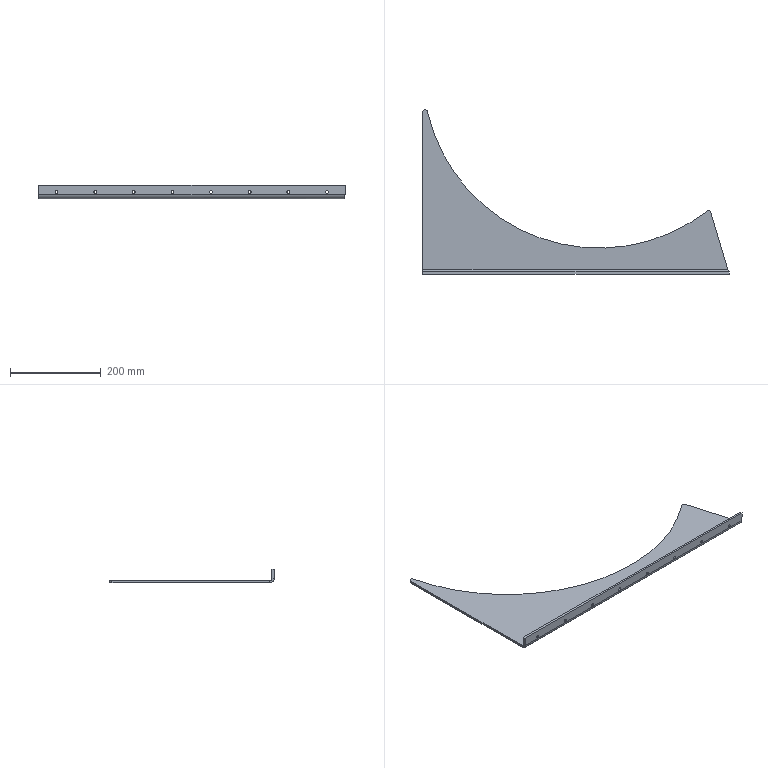Part | SolidWorks | features EdgeFlange 1, Fillet 1, FlatPattern 1, HoleWzd 1, LPattern 1, SMBaseFlange 1, SheetMetal 1 | 1 solid | 48 faces | box 673.852 x 361.966 x 30 mm | volume 462182 mm3 | cylinder 21 | cone 16 | plane 10 | spline 1 | commonest cylinder face diameters 6 x16 10 x3 20 x1 775 x1
STEP:
#1=CARTESIAN_POINT('',(161.352,-444.975,18.));
#2=VERTEX_POINT('',#1);
#3=CARTESIAN_POINT('',(161.352,-444.975,12.));
#4=VERTEX_POINT('',#3);
#5=CARTESIAN_POINT('',(161.352,-444.975,15.));
#6=DIRECTION('',(0.,-1.,0.));
#7=DIRECTION('',(0.,0.,-1.));
#8=AXIS2_PLACEMENT_3D('',#5,#6,#7);
#9=CIRCLE('',#8,3.);
#10=EDGE_CURVE('',#2,#4,#9,.T.);
#11=ORIENTED_EDGE('',*,*,#10,.F.);
#12=CARTESIAN_POINT('',(161.352,-445.,18.025));
#13=VERTEX_POINT('',#12);
#14=CARTESIAN_POINT('',(161.352,-445.,18.025));
#15=DIRECTION('',(0.,-0.7071,0.7071));
#16=VECTOR('',#15,1000.);
#17=LINE('',#14,#16);
#18=EDGE_CURVE('',#2,#13,#17,.T.);
#19=ORIENTED_EDGE('',*,*,#18,.T.);
#20=CARTESIAN_POINT('',(161.352,-445.,11.975));
#21=VERTEX_POINT('',#20);
#22=CARTESIAN_POINT('',(161.352,-445.,15.));
#23=DIRECTION('',(0.,-1.,0.));
#24=DIRECTION('',(0.,0.,-1.));
#25=AXIS2_PLACEMENT_3D('',#22,#23,#24);
#26=CIRCLE('',#25,3.025);
#27=EDGE_CURVE('',#13,#21,#26,.T.);
#28=ORIENTED_EDGE('',*,*,#27,.T.);
#29=CARTESIAN_POINT('',(161.352,-445.,11.975));
#30=DIRECTION('',(0.,-0.7071,-0.7071));
#31=VECTOR('',#30,1000.);
#32=LINE('',#29,#31);
#33=EDGE_CURVE('',#4,#21,#32,.T.);
#34=ORIENTED_EDGE('',*,*,#33,.F.);
#35=EDGE_LOOP('',(#11,#19,#28,#34));
#36=FACE_OUTER_BOUND('',#35,.T.);
#37=CARTESIAN_POINT('',(161.352,-445.,15.));
#38=DIRECTION('',(0.,-1.,0.));
#39=DIRECTION('',(0.,0.,-1.));
#40=AXIS2_PLACEMENT_3D('',#37,#38,#39);
#41=CONICAL_SURFACE('',#40,3.025,0.7854);
#42=ADVANCED_FACE('',(#36),#41,.F.);
#43=CARTESIAN_POINT('',(161.352,-440.,18.));
#44=VERTEX_POINT('',#43);
#45=CARTESIAN_POINT('',(161.352,-440.,12.));
#46=VERTEX_POINT('',#45);
#47=CARTESIAN_POINT('',(161.352,-440.,15.));
#48=DIRECTION('',(0.,-1.,0.));
#49=DIRECTION('',(0.,0.,-1.));
#50=AXIS2_PLACEMENT_3D('',#47,#48,#49);
#51=CIRCLE('',#50,3.);
#52=EDGE_CURVE('',#44,#46,#51,.T.);
#53=ORIENTED_EDGE('',*,*,#52,.F.);
#54=CARTESIAN_POINT('',(161.352,-445.,18.));
#55=DIRECTION('',(0.,-1.,0.));
#56=VECTOR('',#55,1000.);
#57=LINE('',#54,#56);
#58=EDGE_CURVE('',#44,#2,#57,.T.);
#59=ORIENTED_EDGE('',*,*,#58,.T.);
#60=ORIENTED_EDGE('',*,*,#10,.T.);
#61=CARTESIAN_POINT('',(161.352,-445.,12.));
#62=DIRECTION('',(0.,-1.,0.));
#63=VECTOR('',#62,1000.);
#64=LINE('',#61,#63);
#65=EDGE_CURVE('',#46,#4,#64,.T.);
#66=ORIENTED_EDGE('',*,*,#65,.F.);
#67=EDGE_LOOP('',(#53,#59,#60,#66));
#68=FACE_OUTER_BOUND('',#67,.T.);
#69=CARTESIAN_POINT('',(161.352,-445.,15.));
#70=DIRECTION('',(0.,-1.,0.));
#71=DIRECTION('',(0.,0.,-1.));
#72=AXIS2_PLACEMENT_3D('',#69,#70,#71);
#73=CYLINDRICAL_SURFACE('',#72,3.);
#74=ADVANCED_FACE('',(#68),#73,.F.);
#75=CARTESIAN_POINT('',(246.352,-444.975,18.));
#76=VERTEX_POINT('',#75);
#77=CARTESIAN_POINT('',(246.352,-444.975,12.));
#78=VERTEX_POINT('',#77);
#79=CARTESIAN_POINT('',(246.352,-444.975,15.));
#80=DIRECTION('',(0.,-1.,0.));
#81=DIRECTION('',(0.,0.,-1.));
#82=AXIS2_PLACEMENT_3D('',#79,#80,#81);
#83=CIRCLE('',#82,3.);
#84=EDGE_CURVE('',#76,#78,#83,.T.);
#85=ORIENTED_EDGE('',*,*,#84,.F.);
#86=CARTESIAN_POINT('',(246.352,-445.,18.025));
#87=VERTEX_POINT('',#86);
#88=CARTESIAN_POINT('',(246.352,-445.,18.025));
#89=DIRECTION('',(0.,-0.7071,0.7071));
#90=VECTOR('',#89,1000.);
#91=LINE('',#88,#90);
#92=EDGE_CURVE('',#76,#87,#91,.T.);
#93=ORIENTED_EDGE('',*,*,#92,.T.);
#94=CARTESIAN_POINT('',(246.352,-445.,11.975));
#95=VERTEX_POINT('',#94);
#96=CARTESIAN_POINT('',(246.352,-445.,15.));
#97=DIRECTION('',(0.,-1.,0.));
#98=DIRECTION('',(0.,0.,-1.));
#99=AXIS2_PLACEMENT_3D('',#96,#97,#98);
#100=CIRCLE('',#99,3.025);
#101=EDGE_CURVE('',#87,#95,#100,.T.);
#102=ORIENTED_EDGE('',*,*,#101,.T.);
#103=CARTESIAN_POINT('',(246.352,-445.,11.975));
#104=DIRECTION('',(0.,-0.7071,-0.7071));
#105=VECTOR('',#104,1000.);
#106=LINE('',#103,#105);
#107=EDGE_CURVE('',#78,#95,#106,.T.);
#108=ORIENTED_EDGE('',*,*,#107,.F.);
#109=EDGE_LOOP('',(#85,#93,#102,#108));
#110=FACE_OUTER_BOUND('',#109,.T.);
#111=CARTESIAN_POINT('',(246.352,-445.,15.));
#112=DIRECTION('',(0.,-1.,0.));
#113=DIRECTION('',(0.,0.,-1.));
#114=AXIS2_PLACEMENT_3D('',#111,#112,#113);
#115=CONICAL_SURFACE('',#114,3.025,0.7854);
#116=ADVANCED_FACE('',(#110),#115,.F.);
#117=CARTESIAN_POINT('',(246.352,-440.,18.));
#118=VERTEX_POINT('',#117);
#119=CARTESIAN_POINT('',(246.352,-440.,12.));
#120=VERTEX_POINT('',#119);
#121=CARTESIAN_POINT('',(246.352,-440.,15.));
#122=DIRECTION('',(0.,-1.,0.));
#123=DIRECTION('',(0.,0.,-1.));
#124=AXIS2_PLACEMENT_3D('',#121,#122,#123);
#125=CIRCLE('',#124,3.);
#126=EDGE_CURVE('',#118,#120,#125,.T.);
#127=ORIENTED_EDGE('',*,*,#126,.F.);
#128=CARTESIAN_POINT('',(246.352,-445.,18.));
#129=DIRECTION('',(0.,-1.,0.));
#130=VECTOR('',#129,1000.);
#131=LINE('',#128,#130);
#132=EDGE_CURVE('',#118,#76,#131,.T.);
#133=ORIENTED_EDGE('',*,*,#132,.T.);
#134=ORIENTED_EDGE('',*,*,#84,.T.);
#135=CARTESIAN_POINT('',(246.352,-445.,12.));
#136=DIRECTION('',(0.,-1.,0.));
#137=VECTOR('',#136,1000.);
#138=LINE('',#135,#137);
#139=EDGE_CURVE('',#120,#78,#138,.T.);
#140=ORIENTED_EDGE('',*,*,#139,.F.);
#141=EDGE_LOOP('',(#127,#133,#134,#140));
#142=FACE_OUTER_BOUND('',#141,.T.);
#143=CARTESIAN_POINT('',(246.352,-445.,15.));
#144=DIRECTION('',(0.,-1.,0.));
#145=DIRECTION('',(0.,0.,-1.));
#146=AXIS2_PLACEMENT_3D('',#143,#144,#145);
#147=CYLINDRICAL_SURFACE('',#146,3.);
#148=ADVANCED_FACE('',(#142),#147,.F.);
#149=CARTESIAN_POINT('',(76.352,-440.,18.));
#150=VERTEX_POINT('',#149);
#151=CARTESIAN_POINT('',(76.352,-440.,12.));
#152=VERTEX_POINT('',#151);
#153=CARTESIAN_POINT('',(76.352,-440.,15.));
#154=DIRECTION('',(0.,-1.,0.));
#155=DIRECTION('',(0.,0.,-1.));
#156=AXIS2_PLACEMENT_3D('',#153,#154,#155);
#157=CIRCLE('',#156,3.);
#158=EDGE_CURVE('',#150,#152,#157,.T.);
#159=ORIENTED_EDGE('',*,*,#158,.F.);
#160=CARTESIAN_POINT('',(76.352,-444.975,18.));
#161=VERTEX_POINT('',#160);
#162=CARTESIAN_POINT('',(76.352,-445.,18.));
#163=DIRECTION('',(0.,-1.,0.));
#164=VECTOR('',#163,1000.);
#165=LINE('',#162,#164);
#166=EDGE_CURVE('',#150,#161,#165,.T.);
#167=ORIENTED_EDGE('',*,*,#166,.T.);
#168=CARTESIAN_POINT('',(76.352,-444.975,12.));
#169=VERTEX_POINT('',#168);
#170=CARTESIAN_POINT('',(76.352,-444.975,15.));
#171=DIRECTION('',(0.,-1.,0.));
#172=DIRECTION('',(0.,0.,-1.));
#173=AXIS2_PLACEMENT_3D('',#170,#171,#172);
#174=CIRCLE('',#173,3.);
#175=EDGE_CURVE('',#161,#169,#174,.T.);
#176=ORIENTED_EDGE('',*,*,#175,.T.);
#177=CARTESIAN_POINT('',(76.352,-445.,12.));
#178=DIRECTION('',(0.,-1.,0.));
#179=VECTOR('',#178,1000.);
#180=LINE('',#177,#179);
#181=EDGE_CURVE('',#152,#169,#180,.T.);
#182=ORIENTED_EDGE('',*,*,#181,.F.);
#183=EDGE_LOOP('',(#159,#167,#176,#182));
#184=FACE_OUTER_BOUND('',#183,.T.);
#185=CARTESIAN_POINT('',(76.352,-445.,15.));
#186=DIRECTION('',(0.,-1.,0.));
#187=DIRECTION('',(0.,0.,-1.));
#188=AXIS2_PLACEMENT_3D('',#185,#186,#187);
#189=CYLINDRICAL_SURFACE('',#188,3.);
#190=ADVANCED_FACE('',(#184),#189,.F.);
#191=ORIENTED_EDGE('',*,*,#175,.F.);
#192=CARTESIAN_POINT('',(76.352,-445.,18.025));
#193=VERTEX_POINT('',#192);
#194=CARTESIAN_POINT('',(76.352,-445.,18.025));
#195=DIRECTION('',(0.,-0.7071,0.7071));
#196=VECTOR('',#195,1000.);
#197=LINE('',#194,#196);
#198=EDGE_CURVE('',#161,#193,#197,.T.);
#199=ORIENTED_EDGE('',*,*,#198,.T.);
#200=CARTESIAN_POINT('',(76.352,-445.,11.975));
#201=VERTEX_POINT('',#200);
#202=CARTESIAN_POINT('',(76.352,-445.,15.));
#203=DIRECTION('',(0.,-1.,0.));
#204=DIRECTION('',(0.,0.,-1.));
#205=AXIS2_PLACEMENT_3D('',#202,#203,#204);
#206=CIRCLE('',#205,3.025);
#207=EDGE_CURVE('',#193,#201,#206,.T.);
#208=ORIENTED_EDGE('',*,*,#207,.T.);
#209=CARTESIAN_POINT('',(76.352,-445.,11.975));
#210=DIRECTION('',(0.,-0.7071,-0.7071));
#211=VECTOR('',#210,1000.);
#212=LINE('',#209,#211);
#213=EDGE_CURVE('',#169,#201,#212,.T.);
#214=ORIENTED_EDGE('',*,*,#213,.F.);
#215=EDGE_LOOP('',(#191,#199,#208,#214));
#216=FACE_OUTER_BOUND('',#215,.T.);
#217=CARTESIAN_POINT('',(76.352,-445.,15.));
#218=DIRECTION('',(0.,-1.,0.));
#219=DIRECTION('',(0.,0.,-1.));
#220=AXIS2_PLACEMENT_3D('',#217,#218,#219);
#221=CONICAL_SURFACE('',#220,3.025,0.7854);
#222=ADVANCED_FACE('',(#216),#221,.F.);
#223=CARTESIAN_POINT('',(-8.648,-440.,18.));
#224=VERTEX_POINT('',#223);
#225=CARTESIAN_POINT('',(-8.648,-440.,12.));
#226=VERTEX_POINT('',#225);
#227=CARTESIAN_POINT('',(-8.648,-440.,15.));
#228=DIRECTION('',(0.,-1.,0.));
#229=DIRECTION('',(0.,0.,-1.));
#230=AXIS2_PLACEMENT_3D('',#227,#228,#229);
#231=CIRCLE('',#230,3.);
#232=EDGE_CURVE('',#224,#226,#231,.T.);
#233=ORIENTED_EDGE('',*,*,#232,.F.);
#234=CARTESIAN_POINT('',(-8.648,-444.975,18.));
#235=VERTEX_POINT('',#234);
#236=CARTESIAN_POINT('',(-8.648,-445.,18.));
#237=DIRECTION('',(0.,-1.,0.));
#238=VECTOR('',#237,1000.);
#239=LINE('',#236,#238);
#240=EDGE_CURVE('',#224,#235,#239,.T.);
#241=ORIENTED_EDGE('',*,*,#240,.T.);
#242=CARTESIAN_POINT('',(-8.648,-444.975,12.));
#243=VERTEX_POINT('',#242);
#244=CARTESIAN_POINT('',(-8.648,-444.975,15.));
#245=DIRECTION('',(0.,-1.,0.));
#246=DIRECTION('',(0.,0.,-1.));
#247=AXIS2_PLACEMENT_3D('',#244,#245,#246);
#248=CIRCLE('',#247,3.);
#249=EDGE_CURVE('',#235,#243,#248,.T.);
#250=ORIENTED_EDGE('',*,*,#249,.T.);
#251=CARTESIAN_POINT('',(-8.648,-445.,12.));
#252=DIRECTION('',(0.,-1.,0.));
#253=VECTOR('',#252,1000.);
#254=LINE('',#251,#253);
#255=EDGE_CURVE('',#226,#243,#254,.T.);
#256=ORIENTED_EDGE('',*,*,#255,.F.);
#257=EDGE_LOOP('',(#233,#241,#250,#256));
#258=FACE_OUTER_BOUND('',#257,.T.);
#259=CARTESIAN_POINT('',(-8.648,-445.,15.));
#260=DIRECTION('',(0.,-1.,0.));
#261=DIRECTION('',(0.,0.,-1.));
#262=AXIS2_PLACEMENT_3D('',#259,#260,#261);
#263=CYLINDRICAL_SURFACE('',#262,3.);
#264=ADVANCED_FACE('',(#258),#263,.F.);
#265=ORIENTED_EDGE('',*,*,#249,.F.);
#266=CARTESIAN_POINT('',(-8.648,-445.,18.025));
#267=VERTEX_POINT('',#266);
#268=CARTESIAN_POINT('',(-8.648,-445.,18.025));
#269=DIRECTION('',(0.,-0.7071,0.7071));
#270=VECTOR('',#269,1000.);
#271=LINE('',#268,#270);
#272=EDGE_CURVE('',#235,#267,#271,.T.);
#273=ORIENTED_EDGE('',*,*,#272,.T.);
#274=CARTESIAN_POINT('',(-8.648,-445.,11.975));
#275=VERTEX_POINT('',#274);
#276=CARTESIAN_POINT('',(-8.648,-445.,15.));
#277=DIRECTION('',(0.,-1.,0.));
#278=DIRECTION('',(0.,0.,-1.));
#279=AXIS2_PLACEMENT_3D('',#276,#277,#278);
#280=CIRCLE('',#279,3.025);
#281=EDGE_CURVE('',#267,#275,#280,.T.);
#282=ORIENTED_EDGE('',*,*,#281,.T.);
#283=CARTESIAN_POINT('',(-8.648,-445.,11.975));
#284=DIRECTION('',(0.,-0.7071,-0.7071));
#285=VECTOR('',#284,1000.);
#286=LINE('',#283,#285);
#287=EDGE_CURVE('',#243,#275,#286,.T.);
#288=ORIENTED_EDGE('',*,*,#287,.F.);
#289=EDGE_LOOP('',(#265,#273,#282,#288));
#290=FACE_OUTER_BOUND('',#289,.T.);
#291=CARTESIAN_POINT('',(-8.648,-445.,15.));
#292=DIRECTION('',(0.,-1.,0.));
#293=DIRECTION('',(0.,0.,-1.));
#294=AXIS2_PLACEMENT_3D('',#291,#292,#293);
#295=CONICAL_SURFACE('',#294,3.025,0.7854);
#296=ADVANCED_FACE('',(#290),#295,.F.);
#297=CARTESIAN_POINT('',(-93.648,-440.,18.));
#298=VERTEX_POINT('',#297);
#299=CARTESIAN_POINT('',(-93.648,-440.,12.));
#300=VERTEX_POINT('',#299);
#301=CARTESIAN_POINT('',(-93.648,-440.,15.));
#302=DIRECTION('',(0.,-1.,0.));
#303=DIRECTION('',(0.,0.,-1.));
#304=AXIS2_PLACEMENT_3D('',#301,#302,#303);
#305=CIRCLE('',#304,3.);
#306=EDGE_CURVE('',#298,#300,#305,.T.);
#307=ORIENTED_EDGE('',*,*,#306,.F.);
#308=CARTESIAN_POINT('',(-93.648,-444.975,18.));
#309=VERTEX_POINT('',#308);
#310=CARTESIAN_POINT('',(-93.648,-445.,18.));
#311=DIRECTION('',(0.,-1.,0.));
#312=VECTOR('',#311,1000.);
#313=LINE('',#310,#312);
#314=EDGE_CURVE('',#298,#309,#313,.T.);
#315=ORIENTED_EDGE('',*,*,#314,.T.);
#316=CARTESIAN_POINT('',(-93.648,-444.975,12.));
#317=VERTEX_POINT('',#316);
#318=CARTESIAN_POINT('',(-93.648,-444.975,15.));
#319=DIRECTION('',(0.,-1.,0.));
#320=DIRECTION('',(0.,0.,-1.));
#321=AXIS2_PLACEMENT_3D('',#318,#319,#320);
#322=CIRCLE('',#321,3.);
#323=EDGE_CURVE('',#309,#317,#322,.T.);
#324=ORIENTED_EDGE('',*,*,#323,.T.);
#325=CARTESIAN_POINT('',(-93.648,-445.,12.));
#326=DIRECTION('',(0.,-1.,0.));
#327=VECTOR('',#326,1000.);
#328=LINE('',#325,#327);
#329=EDGE_CURVE('',#300,#317,#328,.T.);
#330=ORIENTED_EDGE('',*,*,#329,.F.);
#331=EDGE_LOOP('',(#307,#315,#324,#330));
#332=FACE_OUTER_BOUND('',#331,.T.);
#333=CARTESIAN_POINT('',(-93.648,-445.,15.));
#334=DIRECTION('',(0.,-1.,0.));
#335=DIRECTION('',(0.,0.,-1.));
#336=AXIS2_PLACEMENT_3D('',#333,#334,#335);
#337=CYLINDRICAL_SURFACE('',#336,3.);
#338=ADVANCED_FACE('',(#332),#337,.F.);
#339=ORIENTED_EDGE('',*,*,#323,.F.);
#340=CARTESIAN_POINT('',(-93.648,-445.,18.025));
#341=VERTEX_POINT('',#340);
#342=CARTESIAN_POINT('',(-93.648,-445.,18.025));
#343=DIRECTION('',(0.,-0.7071,0.7071));
#344=VECTOR('',#343,1000.);
#345=LINE('',#342,#344);
#346=EDGE_CURVE('',#309,#341,#345,.T.);
#347=ORIENTED_EDGE('',*,*,#346,.T.);
#348=CARTESIAN_POINT('',(-93.648,-445.,11.975));
#349=VERTEX_POINT('',#348);
#350=CARTESIAN_POINT('',(-93.648,-445.,15.));
#351=DIRECTION('',(0.,-1.,0.));
#352=DIRECTION('',(0.,0.,-1.));
#353=AXIS2_PLACEMENT_3D('',#350,#351,#352);
#354=CIRCLE('',#353,3.025);
#355=EDGE_CURVE('',#341,#349,#354,.T.);
#356=ORIENTED_EDGE('',*,*,#355,.T.);
#357=CARTESIAN_POINT('',(-93.648,-445.,11.975));
#358=DIRECTION('',(0.,-0.7071,-0.7071));
#359=VECTOR('',#358,1000.);
#360=LINE('',#357,#359);
#361=EDGE_CURVE('',#317,#349,#360,.T.);
#362=ORIENTED_EDGE('',*,*,#361,.F.);
#363=EDGE_LOOP('',(#339,#347,#356,#362));
#364=FACE_OUTER_BOUND('',#363,.T.);
#365=CARTESIAN_POINT('',(-93.648,-445.,15.));
#366=DIRECTION('',(0.,-1.,0.));
#367=DIRECTION('',(0.,0.,-1.));
#368=AXIS2_PLACEMENT_3D('',#365,#366,#367);
#369=CONICAL_SURFACE('',#368,3.025,0.7854);
#370=ADVANCED_FACE('',(#364),#369,.F.);
#371=CARTESIAN_POINT('',(-178.648,-440.,18.));
#372=VERTEX_POINT('',#371);
#373=CARTESIAN_POINT('',(-178.648,-440.,12.));
#374=VERTEX_POINT('',#373);
#375=CARTESIAN_POINT('',(-178.648,-440.,15.));
#376=DIRECTION('',(0.,-1.,0.));
#377=DIRECTION('',(0.,0.,-1.));
#378=AXIS2_PLACEMENT_3D('',#375,#376,#377);
#379=CIRCLE('',#378,3.);
#380=EDGE_CURVE('',#372,#374,#379,.T.);
#381=ORIENTED_EDGE('',*,*,#380,.F.);
#382=CARTESIAN_POINT('',(-178.648,-444.975,18.));
#383=VERTEX_POINT('',#382);
#384=CARTESIAN_POINT('',(-178.648,-445.,18.));
#385=DIRECTION('',(0.,-1.,0.));
#386=VECTOR('',#385,1000.);
#387=LINE('',#384,#386);
#388=EDGE_CURVE('',#372,#383,#387,.T.);
#389=ORIENTED_EDGE('',*,*,#388,.T.);
#390=CARTESIAN_POINT('',(-178.648,-444.975,12.));
#391=VERTEX_POINT('',#390);
#392=CARTESIAN_POINT('',(-178.648,-444.975,15.));
#393=DIRECTION('',(0.,-1.,0.));
#394=DIRECTION('',(0.,0.,-1.));
#395=AXIS2_PLACEMENT_3D('',#392,#393,#394);
#396=CIRCLE('',#395,3.);
#397=EDGE_CURVE('',#383,#391,#396,.T.);
#398=ORIENTED_EDGE('',*,*,#397,.T.);
#399=CARTESIAN_POINT('',(-178.648,-445.,12.));
#400=DIRECTION('',(0.,-1.,0.));
#401=VECTOR('',#400,1000.);
#402=LINE('',#399,#401);
#403=EDGE_CURVE('',#374,#391,#402,.T.);
#404=ORIENTED_EDGE('',*,*,#403,.F.);
#405=EDGE_LOOP('',(#381,#389,#398,#404));
#406=FACE_OUTER_BOUND('',#405,.T.);
#407=CARTESIAN_POINT('',(-178.648,-445.,15.));
#408=DIRECTION('',(0.,-1.,0.));
#409=DIRECTION('',(0.,0.,-1.));
#410=AXIS2_PLACEMENT_3D('',#407,#408,#409);
#411=CYLINDRICAL_SURFACE('',#410,3.);
#412=ADVANCED_FACE('',(#406),#411,.F.);
#413=ORIENTED_EDGE('',*,*,#397,.F.);
#414=CARTESIAN_POINT('',(-178.648,-445.,18.025));
#415=VERTEX_POINT('',#414);
#416=CARTESIAN_POINT('',(-178.648,-445.,18.025));
#417=DIRECTION('',(0.,-0.7071,0.7071));
#418=VECTOR('',#417,1000.);
#419=LINE('',#416,#418);
#420=EDGE_CURVE('',#383,#415,#419,.T.);
#421=ORIENTED_EDGE('',*,*,#420,.T.);
#422=CARTESIAN_POINT('',(-178.648,-445.,11.975));
#423=VERTEX_POINT('',#422);
#424=CARTESIAN_POINT('',(-178.648,-445.,15.));
#425=DIRECTION('',(0.,-1.,0.));
#426=DIRECTION('',(0.,0.,-1.));
#427=AXIS2_PLACEMENT_3D('',#424,#425,#426);
#428=CIRCLE('',#427,3.025);
#429=EDGE_CURVE('',#415,#423,#428,.T.);
#430=ORIENTED_EDGE('',*,*,#429,.T.);
#431=CARTESIAN_POINT('',(-178.648,-445.,11.975));
#432=DIRECTION('',(0.,-0.7071,-0.7071));
#433=VECTOR('',#432,1000.);
#434=LINE('',#431,#433);
#435=EDGE_CURVE('',#391,#423,#434,.T.);
#436=ORIENTED_EDGE('',*,*,#435,.F.);
#437=EDGE_LOOP('',(#413,#421,#430,#436));
#438=FACE_OUTER_BOUND('',#437,.T.);
#439=CARTESIAN_POINT('',(-178.648,-445.,15.));
#440=DIRECTION('',(0.,-1.,0.));
#441=DIRECTION('',(0.,0.,-1.));
#442=AXIS2_PLACEMENT_3D('',#439,#440,#441);
#443=CONICAL_SURFACE('',#442,3.025,0.7854);
#444=ADVANCED_FACE('',(#438),#443,.F.);
#445=CARTESIAN_POINT('',(-263.648,-440.,18.));
#446=VERTEX_POINT('',#445);
#447=CARTESIAN_POINT('',(-263.648,-440.,12.));
#448=VERTEX_POINT('',#447);
#449=CARTESIAN_POINT('',(-263.648,-440.,15.));
#450=DIRECTION('',(0.,-1.,0.));
#451=DIRECTION('',(0.,0.,-1.));
#452=AXIS2_PLACEMENT_3D('',#449,#450,#451);
#453=CIRCLE('',#452,3.);
#454=EDGE_CURVE('',#446,#448,#453,.T.);
#455=ORIENTED_EDGE('',*,*,#454,.F.);
#456=CARTESIAN_POINT('',(-263.648,-444.975,18.));
#457=VERTEX_POINT('',#456);
#458=CARTESIAN_POINT('',(-263.648,-445.,18.));
#459=DIRECTION('',(0.,-1.,0.));
#460=VECTOR('',#459,1000.);
#461=LINE('',#458,#460);
#462=EDGE_CURVE('',#446,#457,#461,.T.);
#463=ORIENTED_EDGE('',*,*,#462,.T.);
#464=CARTESIAN_POINT('',(-263.648,-444.975,12.));
#465=VERTEX_POINT('',#464);
#466=CARTESIAN_POINT('',(-263.648,-444.975,15.));
#467=DIRECTION('',(0.,-1.,0.));
#468=DIRECTION('',(0.,0.,-1.));
#469=AXIS2_PLACEMENT_3D('',#466,#467,#468);
#470=CIRCLE('',#469,3.);
#471=EDGE_CURVE('',#457,#465,#470,.T.);
#472=ORIENTED_EDGE('',*,*,#471,.T.);
#473=CARTESIAN_POINT('',(-263.648,-445.,12.));
#474=DIRECTION('',(0.,-1.,0.));
#475=VECTOR('',#474,1000.);
#476=LINE('',#473,#475);
#477=EDGE_CURVE('',#448,#465,#476,.T.);
#478=ORIENTED_EDGE('',*,*,#477,.F.);
#479=EDGE_LOOP('',(#455,#463,#472,#478));
#480=FACE_OUTER_BOUND('',#479,.T.);
#481=CARTESIAN_POINT('',(-263.648,-445.,15.));
#482=DIRECTION('',(0.,-1.,0.));
#483=DIRECTION('',(0.,0.,-1.));
#484=AXIS2_PLACEMENT_3D('',#481,#482,#483);
#485=CYLINDRICAL_SURFACE('',#484,3.);
#486=ADVANCED_FACE('',(#480),#485,.F.);
#487=ORIENTED_EDGE('',*,*,#471,.F.);
#488=CARTESIAN_POINT('',(-263.648,-445.,18.025));
#489=VERTEX_POINT('',#488);
#490=CARTESIAN_POINT('',(-263.648,-445.,18.025));
#491=DIRECTION('',(0.,-0.7071,0.7071));
#492=VECTOR('',#491,1000.);
#493=LINE('',#490,#492);
#494=EDGE_CURVE('',#457,#489,#493,.T.);
#495=ORIENTED_EDGE('',*,*,#494,.T.);
#496=CARTESIAN_POINT('',(-263.648,-445.,11.975));
#497=VERTEX_POINT('',#496);
#498=CARTESIAN_POINT('',(-263.648,-445.,15.));
#499=DIRECTION('',(0.,-1.,0.));
#500=DIRECTION('',(0.,0.,-1.));
#501=AXIS2_PLACEMENT_3D('',#498,#499,#500);
#502=CIRCLE('',#501,3.025);
#503=EDGE_CURVE('',#489,#497,#502,.T.);
#504=ORIENTED_EDGE('',*,*,#503,.T.);
#505=CARTESIAN_POINT('',(-263.648,-445.,11.975));
#506=DIRECTION('',(0.,-0.7071,-0.7071));
#507=VECTOR('',#506,1000.);
#508=LINE('',#505,#507);
#509=EDGE_CURVE('',#465,#497,#508,.T.);
#510=ORIENTED_EDGE('',*,*,#509,.F.);
#511=EDGE_LOOP('',(#487,#495,#504,#510));
#512=FACE_OUTER_BOUND('',#511,.T.);
#513=CARTESIAN_POINT('',(-263.648,-445.,15.));
#514=DIRECTION('',(0.,-1.,0.));
#515=DIRECTION('',(0.,0.,-1.));
#516=AXIS2_PLACEMENT_3D('',#513,#514,#515);
#517=CONICAL_SURFACE('',#516,3.025,0.7854);
#518=ADVANCED_FACE('',(#512),#517,.F.);
#519=CARTESIAN_POINT('',(-348.648,-440.,18.));
#520=VERTEX_POINT('',#519);
#521=CARTESIAN_POINT('',(-348.648,-440.,12.));
#522=VERTEX_POINT('',#521);
#523=CARTESIAN_POINT('',(-348.648,-440.,15.));
#524=DIRECTION('',(0.,-1.,0.));
#525=DIRECTION('',(0.,0.,-1.));
#526=AXIS2_PLACEMENT_3D('',#523,#524,#525);
#527=CIRCLE('',#526,3.);
#528=EDGE_CURVE('',#520,#522,#527,.T.);
#529=ORIENTED_EDGE('',*,*,#528,.F.);
#530=CARTESIAN_POINT('',(-348.648,-444.975,18.));
#531=VERTEX_POINT('',#530);
#532=CARTESIAN_POINT('',(-348.648,-445.,18.));
#533=DIRECTION('',(0.,-1.,0.));
#534=VECTOR('',#533,1000.);
#535=LINE('',#532,#534);
#536=EDGE_CURVE('',#520,#531,#535,.T.);
#537=ORIENTED_EDGE('',*,*,#536,.T.);
#538=CARTESIAN_POINT('',(-348.648,-444.975,12.));
#539=VERTEX_POINT('',#538);
#540=CARTESIAN_POINT('',(-348.648,-444.975,15.));
#541=DIRECTION('',(0.,-1.,0.));
#542=DIRECTION('',(0.,0.,-1.));
#543=AXIS2_PLACEMENT_3D('',#540,#541,#542);
#544=CIRCLE('',#543,3.);
#545=EDGE_CURVE('',#531,#539,#544,.T.);
#546=ORIENTED_EDGE('',*,*,#545,.T.);
#547=CARTESIAN_POINT('',(-348.648,-445.,12.));
#548=DIRECTION('',(0.,-1.,0.));
#549=VECTOR('',#548,1000.);
#550=LINE('',#547,#549);
#551=EDGE_CURVE('',#522,#539,#550,.T.);
#552=ORIENTED_EDGE('',*,*,#551,.F.);
#553=EDGE_LOOP('',(#529,#537,#546,#552));
#554=FACE_OUTER_BOUND('',#553,.T.);
#555=CARTESIAN_POINT('',(-348.648,-445.,15.));
#556=DIRECTION('',(0.,-1.,0.));
#557=DIRECTION('',(0.,0.,-1.));
#558=AXIS2_PLACEMENT_3D('',#555,#556,#557);
#559=CYLINDRICAL_SURFACE('',#558,3.);
#560=ADVANCED_FACE('',(#554),#559,.F.);
#561=ORIENTED_EDGE('',*,*,#545,.F.);
#562=CARTESIAN_POINT('',(-348.648,-445.,18.025));
#563=VERTEX_POINT('',#562);
#564=CARTESIAN_POINT('',(-348.648,-445.,18.025));
#565=DIRECTION('',(0.,-0.7071,0.7071));
#566=VECTOR('',#565,1000.);
#567=LINE('',#564,#566);
#568=EDGE_CURVE('',#531,#563,#567,.T.);
#569=ORIENTED_EDGE('',*,*,#568,.T.);
#570=CARTESIAN_POINT('',(-348.648,-445.,11.975));
#571=VERTEX_POINT('',#570);
#572=CARTESIAN_POINT('',(-348.648,-445.,15.));
#573=DIRECTION('',(0.,-1.,0.));
#574=DIRECTION('',(0.,0.,-1.));
#575=AXIS2_PLACEMENT_3D('',#572,#573,#574);
#576=CIRCLE('',#575,3.025);
#577=EDGE_CURVE('',#563,#571,#576,.T.);
#578=ORIENTED_EDGE('',*,*,#577,.T.);
#579=CARTESIAN_POINT('',(-348.648,-445.,11.975));
#580=DIRECTION('',(0.,-0.7071,-0.7071));
#581=VECTOR('',#580,1000.);
#582=LINE('',#579,#581);
#583=EDGE_CURVE('',#539,#571,#582,.T.);
#584=ORIENTED_EDGE('',*,*,#583,.F.);
#585=EDGE_LOOP('',(#561,#569,#578,#584));
#586=FACE_OUTER_BOUND('',#585,.T.);
#587=CARTESIAN_POINT('',(-348.648,-445.,15.));
#588=DIRECTION('',(0.,-1.,0.));
#589=DIRECTION('',(0.,0.,-1.));
#590=AXIS2_PLACEMENT_3D('',#587,#588,#589);
#591=CONICAL_SURFACE('',#590,3.025,0.7854);
#592=ADVANCED_FACE('',(#586),#591,.F.);
#593=ORIENTED_EDGE('',*,*,#568,.F.);
#594=CARTESIAN_POINT('',(-348.648,-444.975,15.));
#595=DIRECTION('',(0.,-1.,0.));
#596=DIRECTION('',(0.,0.,-1.));
#597=AXIS2_PLACEMENT_3D('',#594,#595,#596);
#598=CIRCLE('',#597,3.);
#599=EDGE_CURVE('',#539,#531,#598,.T.);
#600=ORIENTED_EDGE('',*,*,#599,.F.);
#601=ORIENTED_EDGE('',*,*,#583,.T.);
#602=CARTESIAN_POINT('',(-348.648,-445.,15.));
#603=DIRECTION('',(0.,-1.,0.));
#604=DIRECTION('',(0.,0.,-1.));
#605=AXIS2_PLACEMENT_3D('',#602,#603,#604);
#606=CIRCLE('',#605,3.025);
#607=EDGE_CURVE('',#571,#563,#606,.T.);
#608=ORIENTED_EDGE('',*,*,#607,.T.);
#609=EDGE_LOOP('',(#593,#600,#601,#608));
#610=FACE_OUTER_BOUND('',#609,.T.);
#611=CARTESIAN_POINT('',(-348.648,-445.,15.));
#612=DIRECTION('',(0.,-1.,0.));
#613=DIRECTION('',(0.,0.,-1.));
#614=AXIS2_PLACEMENT_3D('',#611,#612,#613);
#615=CONICAL_SURFACE('',#614,3.025,0.7854);
#616=ADVANCED_FACE('',(#610),#615,.F.);
#617=ORIENTED_EDGE('',*,*,#536,.F.);
#618=CARTESIAN_POINT('',(-348.648,-440.,15.));
#619=DIRECTION('',(0.,-1.,0.));
#620=DIRECTION('',(0.,0.,-1.));
#621=AXIS2_PLACEMENT_3D('',#618,#619,#620);
#622=CIRCLE('',#621,3.);
#623=EDGE_CURVE('',#522,#520,#622,.T.);
#624=ORIENTED_EDGE('',*,*,#623,.F.);
#625=ORIENTED_EDGE('',*,*,#551,.T.);
#626=ORIENTED_EDGE('',*,*,#599,.T.);
#627=EDGE_LOOP('',(#617,#624,#625,#626));
#628=FACE_OUTER_BOUND('',#627,.T.);
#629=CARTESIAN_POINT('',(-348.648,-445.,15.));
#630=DIRECTION('',(0.,-1.,0.));
#631=DIRECTION('',(0.,0.,-1.));
#632=AXIS2_PLACEMENT_3D('',#629,#630,#631);
#633=CYLINDRICAL_SURFACE('',#632,3.);
#634=ADVANCED_FACE('',(#628),#633,.F.);
#635=ORIENTED_EDGE('',*,*,#494,.F.);
#636=CARTESIAN_POINT('',(-263.648,-444.975,15.));
#637=DIRECTION('',(0.,-1.,0.));
#638=DIRECTION('',(0.,0.,-1.));
#639=AXIS2_PLACEMENT_3D('',#636,#637,#638);
#640=CIRCLE('',#639,3.);
#641=EDGE_CURVE('',#465,#457,#640,.T.);
#642=ORIENTED_EDGE('',*,*,#641,.F.);
#643=ORIENTED_EDGE('',*,*,#509,.T.);
#644=CARTESIAN_POINT('',(-263.648,-445.,15.));
#645=DIRECTION('',(0.,-1.,0.));
#646=DIRECTION('',(0.,0.,-1.));
#647=AXIS2_PLACEMENT_3D('',#644,#645,#646);
#648=CIRCLE('',#647,3.025);
#649=EDGE_CURVE('',#497,#489,#648,.T.);
#650=ORIENTED_EDGE('',*,*,#649,.T.);
#651=EDGE_LOOP('',(#635,#642,#643,#650));
#652=FACE_OUTER_BOUND('',#651,.T.);
#653=CARTESIAN_POINT('',(-263.648,-445.,15.));
#654=DIRECTION('',(0.,-1.,0.));
#655=DIRECTION('',(0.,0.,-1.));
#656=AXIS2_PLACEMENT_3D('',#653,#654,#655);
#657=CONICAL_SURFACE('',#656,3.025,0.7854);
#658=ADVANCED_FACE('',(#652),#657,.F.);
#659=ORIENTED_EDGE('',*,*,#462,.F.);
#660=CARTESIAN_POINT('',(-263.648,-440.,15.));
#661=DIRECTION('',(0.,-1.,0.));
#662=DIRECTION('',(0.,0.,-1.));
#663=AXIS2_PLACEMENT_3D('',#660,#661,#662);
#664=CIRCLE('',#663,3.);
#665=EDGE_CURVE('',#448,#446,#664,.T.);
#666=ORIENTED_EDGE('',*,*,#665,.F.);
#667=ORIENTED_EDGE('',*,*,#477,.T.);
#668=ORIENTED_EDGE('',*,*,#641,.T.);
#669=EDGE_LOOP('',(#659,#666,#667,#668));
#670=FACE_OUTER_BOUND('',#669,.T.);
#671=CARTESIAN_POINT('',(-263.648,-445.,15.));
#672=DIRECTION('',(0.,-1.,0.));
#673=DIRECTION('',(0.,0.,-1.));
#674=AXIS2_PLACEMENT_3D('',#671,#672,#673);
#675=CYLINDRICAL_SURFACE('',#674,3.);
#676=ADVANCED_FACE('',(#670),#675,.F.);
#677=ORIENTED_EDGE('',*,*,#420,.F.);
#678=CARTESIAN_POINT('',(-178.648,-444.975,15.));
#679=DIRECTION('',(0.,-1.,0.));
#680=DIRECTION('',(0.,0.,-1.));
#681=AXIS2_PLACEMENT_3D('',#678,#679,#680);
#682=CIRCLE('',#681,3.);
#683=EDGE_CURVE('',#391,#383,#682,.T.);
#684=ORIENTED_EDGE('',*,*,#683,.F.);
#685=ORIENTED_EDGE('',*,*,#435,.T.);
#686=CARTESIAN_POINT('',(-178.648,-445.,15.));
#687=DIRECTION('',(0.,-1.,0.));
#688=DIRECTION('',(0.,0.,-1.));
#689=AXIS2_PLACEMENT_3D('',#686,#687,#688);
#690=CIRCLE('',#689,3.025);
#691=EDGE_CURVE('',#423,#415,#690,.T.);
#692=ORIENTED_EDGE('',*,*,#691,.T.);
#693=EDGE_LOOP('',(#677,#684,#685,#692));
#694=FACE_OUTER_BOUND('',#693,.T.);
#695=CARTESIAN_POINT('',(-178.648,-445.,15.));
#696=DIRECTION('',(0.,-1.,0.));
#697=DIRECTION('',(0.,0.,-1.));
#698=AXIS2_PLACEMENT_3D('',#695,#696,#697);
#699=CONICAL_SURFACE('',#698,3.025,0.7854);
#700=ADVANCED_FACE('',(#694),#699,.F.);
#701=ORIENTED_EDGE('',*,*,#388,.F.);
#702=CARTESIAN_POINT('',(-178.648,-440.,15.));
#703=DIRECTION('',(0.,-1.,0.));
#704=DIRECTION('',(0.,0.,-1.));
#705=AXIS2_PLACEMENT_3D('',#702,#703,#704);
#706=CIRCLE('',#705,3.);
#707=EDGE_CURVE('',#374,#372,#706,.T.);
#708=ORIENTED_EDGE('',*,*,#707,.F.);
#709=ORIENTED_EDGE('',*,*,#403,.T.);
#710=ORIENTED_EDGE('',*,*,#683,.T.);
#711=EDGE_LOOP('',(#701,#708,#709,#710));
#712=FACE_OUTER_BOUND('',#711,.T.);
#713=CARTESIAN_POINT('',(-178.648,-445.,15.));
#714=DIRECTION('',(0.,-1.,0.));
#715=DIRECTION('',(0.,0.,-1.));
#716=AXIS2_PLACEMENT_3D('',#713,#714,#715);
#717=CYLINDRICAL_SURFACE('',#716,3.);
#718=ADVANCED_FACE('',(#712),#717,.F.);
#719=ORIENTED_EDGE('',*,*,#346,.F.);
#720=CARTESIAN_POINT('',(-93.648,-444.975,15.));
#721=DIRECTION('',(0.,-1.,0.));
#722=DIRECTION('',(0.,0.,-1.));
#723=AXIS2_PLACEMENT_3D('',#720,#721,#722);
#724=CIRCLE('',#723,3.);
#725=EDGE_CURVE('',#317,#309,#724,.T.);
#726=ORIENTED_EDGE('',*,*,#725,.F.);
#727=ORIENTED_EDGE('',*,*,#361,.T.);
#728=CARTESIAN_POINT('',(-93.648,-445.,15.));
#729=DIRECTION('',(0.,-1.,0.));
#730=DIRECTION('',(0.,0.,-1.));
#731=AXIS2_PLACEMENT_3D('',#728,#729,#730);
#732=CIRCLE('',#731,3.025);
#733=EDGE_CURVE('',#349,#341,#732,.T.);
#734=ORIENTED_EDGE('',*,*,#733,.T.);
#735=EDGE_LOOP('',(#719,#726,#727,#734));
#736=FACE_OUTER_BOUND('',#735,.T.);
#737=CARTESIAN_POINT('',(-93.648,-445.,15.));
#738=DIRECTION('',(0.,-1.,0.));
#739=DIRECTION('',(0.,0.,-1.));
#740=AXIS2_PLACEMENT_3D('',#737,#738,#739);
#741=CONICAL_SURFACE('',#740,3.025,0.7854);
#742=ADVANCED_FACE('',(#736),#741,.F.);
#743=ORIENTED_EDGE('',*,*,#314,.F.);
#744=CARTESIAN_POINT('',(-93.648,-440.,15.));
#745=DIRECTION('',(0.,-1.,0.));
#746=DIRECTION('',(0.,0.,-1.));
#747=AXIS2_PLACEMENT_3D('',#744,#745,#746);
#748=CIRCLE('',#747,3.);
#749=EDGE_CURVE('',#300,#298,#748,.T.);
#750=ORIENTED_EDGE('',*,*,#749,.F.);
#751=ORIENTED_EDGE('',*,*,#329,.T.);
#752=ORIENTED_EDGE('',*,*,#725,.T.);
#753=EDGE_LOOP('',(#743,#750,#751,#752));
#754=FACE_OUTER_BOUND('',#753,.T.);
#755=CARTESIAN_POINT('',(-93.648,-445.,15.));
#756=DIRECTION('',(0.,-1.,0.));
#757=DIRECTION('',(0.,0.,-1.));
#758=AXIS2_PLACEMENT_3D('',#755,#756,#757);
#759=CYLINDRICAL_SURFACE('',#758,3.);
#760=ADVANCED_FACE('',(#754),#759,.F.);
#761=ORIENTED_EDGE('',*,*,#272,.F.);
#762=CARTESIAN_POINT('',(-8.648,-444.975,15.));
#763=DIRECTION('',(0.,-1.,0.));
#764=DIRECTION('',(0.,0.,-1.));
#765=AXIS2_PLACEMENT_3D('',#762,#763,#764);
#766=CIRCLE('',#765,3.);
#767=EDGE_CURVE('',#243,#235,#766,.T.);
#768=ORIENTED_EDGE('',*,*,#767,.F.);
#769=ORIENTED_EDGE('',*,*,#287,.T.);
#770=CARTESIAN_POINT('',(-8.648,-445.,15.));
#771=DIRECTION('',(0.,-1.,0.));
#772=DIRECTION('',(0.,0.,-1.));
#773=AXIS2_PLACEMENT_3D('',#770,#771,#772);
#774=CIRCLE('',#773,3.025);
#775=EDGE_CURVE('',#275,#267,#774,.T.);
#776=ORIENTED_EDGE('',*,*,#775,.T.);
#777=EDGE_LOOP('',(#761,#768,#769,#776));
#778=FACE_OUTER_BOUND('',#777,.T.);
#779=CARTESIAN_POINT('',(-8.648,-445.,15.));
#780=DIRECTION('',(0.,-1.,0.));
#781=DIRECTION('',(0.,0.,-1.));
#782=AXIS2_PLACEMENT_3D('',#779,#780,#781);
#783=CONICAL_SURFACE('',#782,3.025,0.7854);
#784=ADVANCED_FACE('',(#778),#783,.F.);
#785=ORIENTED_EDGE('',*,*,#240,.F.);
#786=CARTESIAN_POINT('',(-8.648,-440.,15.));
#787=DIRECTION('',(0.,-1.,0.));
#788=DIRECTION('',(0.,0.,-1.));
#789=AXIS2_PLACEMENT_3D('',#786,#787,#788);
#790=CIRCLE('',#789,3.);
#791=EDGE_CURVE('',#226,#224,#790,.T.);
#792=ORIENTED_EDGE('',*,*,#791,.F.);
#793=ORIENTED_EDGE('',*,*,#255,.T.);
#794=ORIENTED_EDGE('',*,*,#767,.T.);
#795=EDGE_LOOP('',(#785,#792,#793,#794));
#796=FACE_OUTER_BOUND('',#795,.T.);
#797=CARTESIAN_POINT('',(-8.648,-445.,15.));
#798=DIRECTION('',(0.,-1.,0.));
#799=DIRECTION('',(0.,0.,-1.));
#800=AXIS2_PLACEMENT_3D('',#797,#798,#799);
#801=CYLINDRICAL_SURFACE('',#800,3.);
#802=ADVANCED_FACE('',(#796),#801,.F.);
#803=ORIENTED_EDGE('',*,*,#198,.F.);
#804=CARTESIAN_POINT('',(76.352,-444.975,15.));
#805=DIRECTION('',(0.,-1.,0.));
#806=DIRECTION('',(0.,0.,-1.));
#807=AXIS2_PLACEMENT_3D('',#804,#805,#806);
#808=CIRCLE('',#807,3.);
#809=EDGE_CURVE('',#169,#161,#808,.T.);
#810=ORIENTED_EDGE('',*,*,#809,.F.);
#811=ORIENTED_EDGE('',*,*,#213,.T.);
#812=CARTESIAN_POINT('',(76.352,-445.,15.));
#813=DIRECTION('',(0.,-1.,0.));
#814=DIRECTION('',(0.,0.,-1.));
#815=AXIS2_PLACEMENT_3D('',#812,#813,#814);
#816=CIRCLE('',#815,3.025);
#817=EDGE_CURVE('',#201,#193,#816,.T.);
#818=ORIENTED_EDGE('',*,*,#817,.T.);
#819=EDGE_LOOP('',(#803,#810,#811,#818));
#820=FACE_OUTER_BOUND('',#819,.T.);
#821=CARTESIAN_POINT('',(76.352,-445.,15.));
#822=DIRECTION('',(0.,-1.,0.));
#823=DIRECTION('',(0.,0.,-1.));
#824=AXIS2_PLACEMENT_3D('',#821,#822,#823);
#825=CONICAL_SURFACE('',#824,3.025,0.7854);
#826=ADVANCED_FACE('',(#820),#825,.F.);
#827=ORIENTED_EDGE('',*,*,#166,.F.);
#828=CARTESIAN_POINT('',(76.352,-440.,15.));
#829=DIRECTION('',(0.,-1.,0.));
#830=DIRECTION('',(0.,0.,-1.));
#831=AXIS2_PLACEMENT_3D('',#828,#829,#830);
#832=CIRCLE('',#831,3.);
#833=EDGE_CURVE('',#152,#150,#832,.T.);
#834=ORIENTED_EDGE('',*,*,#833,.F.);
#835=ORIENTED_EDGE('',*,*,#181,.T.);
#836=ORIENTED_EDGE('',*,*,#809,.T.);
#837=EDGE_LOOP('',(#827,#834,#835,#836));
#838=FACE_OUTER_BOUND('',#837,.T.);
#839=CARTESIAN_POINT('',(76.352,-445.,15.));
#840=DIRECTION('',(0.,-1.,0.));
#841=DIRECTION('',(0.,0.,-1.));
#842=AXIS2_PLACEMENT_3D('',#839,#840,#841);
#843=CYLINDRICAL_SURFACE('',#842,3.);
#844=ADVANCED_FACE('',(#838),#843,.F.);
#845=CARTESIAN_POINT('',(283.399,-435.,0.));
#846=VERTEX_POINT('',#845);
#847=CARTESIAN_POINT('',(245.961,-308.253,0.));
#848=VERTEX_POINT('',#847);
#849=CARTESIAN_POINT('',(243.862,-301.144,0.));
#850=DIRECTION('',(-0.2833,0.959,0.));
#851=VECTOR('',#850,1000.);
#852=LINE('',#849,#851);
#853=EDGE_CURVE('',#846,#848,#852,.T.);
#854=ORIENTED_EDGE('',*,*,#853,.T.);
#855=CARTESIAN_POINT('',(245.961,-308.253,5.));
#856=VERTEX_POINT('',#855);
#857=CARTESIAN_POINT('',(245.961,-308.253,5.));
#858=DIRECTION('',(0.,0.,1.));
#859=VECTOR('',#858,1000.);
#860=LINE('',#857,#859);
#861=EDGE_CURVE('',#848,#856,#860,.T.);
#862=ORIENTED_EDGE('',*,*,#861,.T.);
#863=CARTESIAN_POINT('',(283.399,-435.,5.));
#864=VERTEX_POINT('',#863);
#865=CARTESIAN_POINT('',(243.862,-301.144,5.));
#866=DIRECTION('',(-0.2833,0.959,0.));
#867=VECTOR('',#866,1000.);
#868=LINE('',#865,#867);
#869=EDGE_CURVE('',#864,#856,#868,.T.);
#870=ORIENTED_EDGE('',*,*,#869,.F.);
#871=CARTESIAN_POINT('',(283.399,-435.,5.));
#872=DIRECTION('',(0.,0.,-1.));
#873=VECTOR('',#872,1000.);
#874=LINE('',#871,#873);
#875=EDGE_CURVE('',#864,#846,#874,.T.);
#876=ORIENTED_EDGE('',*,*,#875,.T.);
#877=EDGE_LOOP('',(#854,#862,#870,#876));
#878=FACE_OUTER_BOUND('',#877,.T.);
#879=CARTESIAN_POINT('',(243.862,-301.144,5.));
#880=DIRECTION('',(-0.959,-0.2833,0.));
#881=DIRECTION('',(0.2833,-0.959,0.));
#882=AXIS2_PLACEMENT_3D('',#879,#880,#881);
#883=PLANE('',#882);
#884=ADVANCED_FACE('',(#878),#883,.F.);
#885=CARTESIAN_POINT('',(-387.5,-88.034,5.));
#886=VERTEX_POINT('',#885);
#887=CARTESIAN_POINT('',(-387.5,-435.,5.));
#888=VERTEX_POINT('',#887);
#889=CARTESIAN_POINT('',(-387.5,0.,5.));
#890=DIRECTION('',(0.,-1.,0.));
#891=VECTOR('',#890,1000.);
#892=LINE('',#889,#891);
#893=EDGE_CURVE('',#886,#888,#892,.T.);
#894=ORIENTED_EDGE('',*,*,#893,.F.);
#895=CARTESIAN_POINT('',(-387.5,-88.034,0.));
#896=VERTEX_POINT('',#895);
#897=CARTESIAN_POINT('',(-387.5,-88.034,5.));
#898=DIRECTION('',(0.,0.,-1.));
#899=VECTOR('',#898,1000.);
#900=LINE('',#897,#899);
#901=EDGE_CURVE('',#886,#896,#900,.T.);
#902=ORIENTED_EDGE('',*,*,#901,.T.);
#903=CARTESIAN_POINT('',(-387.5,-435.,0.));
#904=VERTEX_POINT('',#903);
#905=CARTESIAN_POINT('',(-387.5,0.,0.));
#906=DIRECTION('',(0.,-1.,0.));
#907=VECTOR('',#906,1000.);
#908=LINE('',#905,#907);
#909=EDGE_CURVE('',#896,#904,#908,.T.);
#910=ORIENTED_EDGE('',*,*,#909,.T.);
#911=CARTESIAN_POINT('',(-387.5,-435.,5.));
#912=DIRECTION('',(0.,0.,-1.));
#913=VECTOR('',#912,1000.);
#914=LINE('',#911,#913);
#915=EDGE_CURVE('',#888,#904,#914,.T.);
#916=ORIENTED_EDGE('',*,*,#915,.F.);
#917=EDGE_LOOP('',(#894,#902,#910,#916));
#918=FACE_OUTER_BOUND('',#917,.T.);
#919=CARTESIAN_POINT('',(-387.5,0.,5.));
#920=DIRECTION('',(1.,0.,0.));
#921=DIRECTION('',(0.,1.,0.));
#922=AXIS2_PLACEMENT_3D('',#919,#920,#921);
#923=PLANE('',#922);
#924=ADVANCED_FACE('',(#918),#923,.F.);
#925=ORIENTED_EDGE('',*,*,#869,.T.);
#926=CARTESIAN_POINT('',(238.094,-305.725,5.));
#927=VERTEX_POINT('',#926);
#928=CARTESIAN_POINT('',(241.166,-309.669,5.));
#929=DIRECTION('',(0.,0.,1.));
#930=DIRECTION('',(1.,0.,0.));
#931=AXIS2_PLACEMENT_3D('',#928,#929,#930);
#932=CIRCLE('',#931,5.);
#933=EDGE_CURVE('',#856,#927,#932,.T.);
#934=ORIENTED_EDGE('',*,*,#933,.T.);
#935=CARTESIAN_POINT('',(-377.627,-86.913,5.));
#936=VERTEX_POINT('',#935);
#937=CARTESIAN_POINT('',(0.,0.,5.));
#938=DIRECTION('',(0.,0.,-1.));
#939=DIRECTION('',(1.,0.,0.));
#940=AXIS2_PLACEMENT_3D('',#937,#938,#939);
#941=CIRCLE('',#940,387.5);
#942=EDGE_CURVE('',#927,#936,#941,.T.);
#943=ORIENTED_EDGE('',*,*,#942,.T.);
#944=CARTESIAN_POINT('',(-382.5,-88.034,5.));
#945=DIRECTION('',(0.,0.,1.));
#946=DIRECTION('',(1.,0.,0.));
#947=AXIS2_PLACEMENT_3D('',#944,#945,#946);
#948=CIRCLE('',#947,5.);
#949=EDGE_CURVE('',#936,#886,#948,.T.);
#950=ORIENTED_EDGE('',*,*,#949,.T.);
#951=ORIENTED_EDGE('',*,*,#893,.T.);
#952=CARTESIAN_POINT('',(286.352,-435.,5.));
#953=DIRECTION('',(-1.,0.,0.));
#954=VECTOR('',#953,1000.);
#955=LINE('',#952,#954);
#956=EDGE_CURVE('',#864,#888,#955,.T.);
#957=ORIENTED_EDGE('',*,*,#956,.F.);
#958=EDGE_LOOP('',(#925,#934,#943,#950,#951,#957));
#959=FACE_OUTER_BOUND('',#958,.T.);
#960=CARTESIAN_POINT('',(0.,0.,5.));
#961=DIRECTION('',(0.,0.,1.));
#962=DIRECTION('',(1.,0.,0.));
#963=AXIS2_PLACEMENT_3D('',#960,#961,#962);
#964=PLANE('',#963);
#965=ADVANCED_FACE('',(#959),#964,.T.);
#966=CARTESIAN_POINT('',(238.094,-305.725,0.));
#967=VERTEX_POINT('',#966);
#968=CARTESIAN_POINT('',(-377.627,-86.913,0.));
#969=VERTEX_POINT('',#968);
#970=CARTESIAN_POINT('',(0.,0.,0.));
#971=DIRECTION('',(0.,0.,-1.));
#972=DIRECTION('',(1.,0.,0.));
#973=AXIS2_PLACEMENT_3D('',#970,#971,#972);
#974=CIRCLE('',#973,387.5);
#975=EDGE_CURVE('',#967,#969,#974,.T.);
#976=ORIENTED_EDGE('',*,*,#975,.F.);
#977=CARTESIAN_POINT('',(241.166,-309.669,0.));
#978=DIRECTION('',(0.,0.,-1.));
#979=DIRECTION('',(1.,0.,0.));
#980=AXIS2_PLACEMENT_3D('',#977,#978,#979);
#981=CIRCLE('',#980,5.);
#982=EDGE_CURVE('',#967,#848,#981,.T.);
#983=ORIENTED_EDGE('',*,*,#982,.T.);
#984=ORIENTED_EDGE('',*,*,#853,.F.);
#985=CARTESIAN_POINT('',(286.352,-435.,0.));
#986=DIRECTION('',(-1.,0.,0.));
#987=VECTOR('',#986,1000.);
#988=LINE('',#985,#987);
#989=EDGE_CURVE('',#846,#904,#988,.T.);
#990=ORIENTED_EDGE('',*,*,#989,.T.);
#991=ORIENTED_EDGE('',*,*,#909,.F.);
#992=CARTESIAN_POINT('',(-382.5,-88.034,0.));
#993=DIRECTION('',(0.,0.,-1.));
#994=DIRECTION('',(1.,0.,0.));
#995=AXIS2_PLACEMENT_3D('',#992,#993,#994);
#996=CIRCLE('',#995,5.);
#997=EDGE_CURVE('',#896,#969,#996,.T.);
#998=ORIENTED_EDGE('',*,*,#997,.T.);
#999=EDGE_LOOP('',(#976,#983,#984,#990,#991,#998));
#1000=FACE_OUTER_BOUND('',#999,.T.);
#1001=CARTESIAN_POINT('',(0.,0.,0.));
#1002=DIRECTION('',(0.,0.,1.));
#1003=DIRECTION('',(1.,0.,0.));
#1004=AXIS2_PLACEMENT_3D('',#1001,#1002,#1003);
#1005=PLANE('',#1004);
#1006=ADVANCED_FACE('',(#1000),#1005,.F.);
#1007=ORIENTED_EDGE('',*,*,#942,.F.);
#1008=CARTESIAN_POINT('',(238.094,-305.725,5.));
#1009=DIRECTION('',(0.,0.,-1.));
#1010=VECTOR('',#1009,1000.);
#1011=LINE('',#1008,#1010);
#1012=EDGE_CURVE('',#927,#967,#1011,.T.);
#1013=ORIENTED_EDGE('',*,*,#1012,.T.);
#1014=ORIENTED_EDGE('',*,*,#975,.T.);
#1015=CARTESIAN_POINT('',(-377.627,-86.913,5.));
#1016=DIRECTION('',(0.,0.,1.));
#1017=VECTOR('',#1016,1000.);
#1018=LINE('',#1015,#1017);
#1019=EDGE_CURVE('',#969,#936,#1018,.T.);
#1020=ORIENTED_EDGE('',*,*,#1019,.T.);
#1021=EDGE_LOOP('',(#1007,#1013,#1014,#1020));
#1022=FACE_OUTER_BOUND('',#1021,.T.);
#1023=CARTESIAN_POINT('',(0.,0.,5.));
#1024=DIRECTION('',(0.,0.,-1.));
#1025=DIRECTION('',(-1.,0.,0.));
#1026=AXIS2_PLACEMENT_3D('',#1023,#1024,#1025);
#1027=CYLINDRICAL_SURFACE('',#1026,387.5);
#1028=ADVANCED_FACE('',(#1022),#1027,.F.);
#1029=CARTESIAN_POINT('',(-387.5,-440.,10.));
#1030=VERTEX_POINT('',#1029);
#1031=CARTESIAN_POINT('',(-387.5,-445.,10.));
#1032=VERTEX_POINT('',#1031);
#1033=CARTESIAN_POINT('',(-387.5,-445.,10.));
#1034=DIRECTION('',(0.,-1.,0.));
#1035=VECTOR('',#1034,1000.);
#1036=LINE('',#1033,#1035);
#1037=EDGE_CURVE('',#1030,#1032,#1036,.T.);
#1038=ORIENTED_EDGE('',*,*,#1037,.F.);
#1039=CARTESIAN_POINT('',(-387.5,-435.,10.));
#1040=DIRECTION('',(-1.,0.,0.));
#1041=DIRECTION('',(0.,0.,-1.));
#1042=AXIS2_PLACEMENT_3D('',#1039,#1040,#1041);
#1043=CIRCLE('',#1042,5.);
#1044=EDGE_CURVE('',#888,#1030,#1043,.T.);
#1045=ORIENTED_EDGE('',*,*,#1044,.F.);
#1046=ORIENTED_EDGE('',*,*,#915,.T.);
#1047=CARTESIAN_POINT('',(-387.5,-435.,10.));
#1048=DIRECTION('',(-1.,0.,0.));
#1049=DIRECTION('',(0.,0.,-1.));
#1050=AXIS2_PLACEMENT_3D('',#1047,#1048,#1049);
#1051=CIRCLE('',#1050,10.);
#1052=EDGE_CURVE('',#904,#1032,#1051,.T.);
#1053=ORIENTED_EDGE('',*,*,#1052,.T.);
#1054=EDGE_LOOP('',(#1038,#1045,#1046,#1053));
#1055=FACE_OUTER_BOUND('',#1054,.T.);
#1056=CARTESIAN_POINT('',(-387.5,-435.,10.));
#1057=DIRECTION('',(-1.,0.,0.));
#1058=DIRECTION('',(0.,0.,1.));
#1059=AXIS2_PLACEMENT_3D('',#1056,#1057,#1058);
#1060=PLANE('',#1059);
#1061=ADVANCED_FACE('',(#1055),#1060,.T.);
#1062=CARTESIAN_POINT('',(286.352,-440.,10.));
#1063=VERTEX_POINT('',#1062);
#1064=CARTESIAN_POINT('',(286.352,-440.,10.));
#1065=CARTESIAN_POINT('',(286.228,-440.,9.67));
#1066=CARTESIAN_POINT('',(286.106,-439.968,9.345));
#1067=CARTESIAN_POINT('',(285.861,-439.841,8.706));
#1068=CARTESIAN_POINT('',(285.738,-439.745,8.39));
#1069=CARTESIAN_POINT('',(285.491,-439.494,7.783));
#1070=CARTESIAN_POINT('',(285.368,-439.34,7.496));
#1071=CARTESIAN_POINT('',(285.123,-438.978,6.954));
#1072=CARTESIAN_POINT('',(284.999,-438.768,6.697));
#1073=CARTESIAN_POINT('',(284.753,-438.305,6.234));
#1074=CARTESIAN_POINT('',(284.631,-438.053,6.027));
#1075=CARTESIAN_POINT('',(284.385,-437.511,5.664));
#1076=CARTESIAN_POINT('',(284.261,-437.217,5.507));
#1077=CARTESIAN_POINT('',(284.015,-436.614,5.256));
#1078=CARTESIAN_POINT('',(283.893,-436.303,5.162));
#1079=CARTESIAN_POINT('',(283.647,-435.661,5.033));
#1080=CARTESIAN_POINT('',(283.523,-435.33,5.));
#1081=CARTESIAN_POINT('',(283.399,-435.,5.));
#1082=B_SPLINE_CURVE_WITH_KNOTS('',3,(#1064,#1065,#1066,#1067,#1068,#1069,#1070,#1071,#1072,#1073,#1074,#1075,#1076,#1077,#1078,#1079,#1080,#1081),.UNSPECIFIED.,.F.,.F.,(4,2,2,2,2,2,2,2,4),(0.,0.001043,0.002086,0.00313,0.004173,0.005216,0.006259,0.007302,0.008346),.UNSPECIFIED.);
#1083=EDGE_CURVE('',#1063,#864,#1082,.T.);
#1084=ORIENTED_EDGE('',*,*,#1083,.F.);
#1085=CARTESIAN_POINT('',(286.352,-445.,10.));
#1086=VERTEX_POINT('',#1085);
#1087=CARTESIAN_POINT('',(286.352,-440.,10.));
#1088=DIRECTION('',(0.,-1.,0.));
#1089=VECTOR('',#1088,1000.);
#1090=LINE('',#1087,#1089);
#1091=EDGE_CURVE('',#1063,#1086,#1090,.T.);
#1092=ORIENTED_EDGE('',*,*,#1091,.T.);
#1093=CARTESIAN_POINT('',(286.352,-445.,10.));
#1094=CARTESIAN_POINT('',(286.228,-445.,9.34));
#1095=CARTESIAN_POINT('',(286.106,-444.935,8.69));
#1096=CARTESIAN_POINT('',(285.923,-444.745,7.732));
#1097=CARTESIAN_POINT('',(285.861,-444.666,7.416));
#1098=CARTESIAN_POINT('',(285.738,-444.476,6.788));
#1099=CARTESIAN_POINT('',(285.676,-444.364,6.476));
#1100=CARTESIAN_POINT('',(285.491,-443.988,5.568));
#1101=CARTESIAN_POINT('',(285.369,-443.681,4.993));
#1102=CARTESIAN_POINT('',(285.124,-442.957,3.908));
#1103=CARTESIAN_POINT('',(284.999,-442.535,3.393));
#1104=CARTESIAN_POINT('',(284.754,-441.612,2.47));
#1105=CARTESIAN_POINT('',(284.632,-441.109,2.056));
#1106=CARTESIAN_POINT('',(284.447,-440.292,1.509));
#1107=CARTESIAN_POINT('',(284.385,-440.008,1.338));
#1108=CARTESIAN_POINT('',(284.261,-439.43,1.029));
#1109=CARTESIAN_POINT('',(284.2,-439.135,0.8892));
#1110=CARTESIAN_POINT('',(284.016,-438.233,0.5147));
#1111=CARTESIAN_POINT('',(283.894,-437.609,0.3238));
#1112=CARTESIAN_POINT('',(283.646,-436.314,0.06478));
#1113=CARTESIAN_POINT('',(283.523,-435.66,0.));
#1114=CARTESIAN_POINT('',(283.399,-435.,0.));
#1115=B_SPLINE_CURVE_WITH_KNOTS('',3,(#1093,#1094,#1095,#1096,#1097,#1098,#1099,#1100,#1101,#1102,#1103,#1104,#1105,#1106,#1107,#1108,#1109,#1110,#1111,#1112,#1113,#1114),.UNSPECIFIED.,.F.,.F.,(4,2,2,2,2,2,2,2,2,2,4),(0.,0.001987,0.00298,0.003974,0.005961,0.007947,0.009934,0.01093,0.01192,0.01391,0.01589),.UNSPECIFIED.);
#1116=EDGE_CURVE('',#1086,#846,#1115,.T.);
#1117=ORIENTED_EDGE('',*,*,#1116,.T.);
#1118=ORIENTED_EDGE('',*,*,#875,.F.);
#1119=EDGE_LOOP('',(#1084,#1092,#1117,#1118));
#1120=FACE_OUTER_BOUND('',#1119,.T.);
#1121=CARTESIAN_POINT('',(286.352,-445.05,10.));
#1122=CARTESIAN_POINT('',(286.106,-445.05,8.684));
#1123=CARTESIAN_POINT('',(285.86,-444.788,7.369));
#1124=CARTESIAN_POINT('',(285.368,-443.782,4.939));
#1125=CARTESIAN_POINT('',(285.122,-443.037,3.824));
#1126=CARTESIAN_POINT('',(284.629,-441.176,1.963));
#1127=CARTESIAN_POINT('',(284.383,-440.061,1.218));
#1128=CARTESIAN_POINT('',(283.891,-437.631,0.2116));
#1129=CARTESIAN_POINT('',(283.645,-436.316,-0.05));
#1130=CARTESIAN_POINT('',(283.399,-435.,-0.05));
#1131=CARTESIAN_POINT('',(286.352,-445.,10.));
#1132=CARTESIAN_POINT('',(286.106,-445.,8.691));
#1133=CARTESIAN_POINT('',(285.86,-444.74,7.383));
#1134=CARTESIAN_POINT('',(285.368,-443.738,4.964));
#1135=CARTESIAN_POINT('',(285.122,-442.997,3.855));
#1136=CARTESIAN_POINT('',(284.629,-441.145,2.003));
#1137=CARTESIAN_POINT('',(284.383,-440.036,1.262));
#1138=CARTESIAN_POINT('',(283.891,-437.617,0.2603));
#1139=CARTESIAN_POINT('',(283.645,-436.309,0.));
#1140=CARTESIAN_POINT('',(283.399,-435.,0.));
#1141=CARTESIAN_POINT('',(286.352,-440.,10.));
#1142=CARTESIAN_POINT('',(286.106,-440.,9.345));
#1143=CARTESIAN_POINT('',(285.86,-439.87,8.691));
#1144=CARTESIAN_POINT('',(285.368,-439.369,7.482));
#1145=CARTESIAN_POINT('',(285.122,-438.998,6.927));
#1146=CARTESIAN_POINT('',(284.629,-438.073,6.002));
#1147=CARTESIAN_POINT('',(284.383,-437.518,5.631));
#1148=CARTESIAN_POINT('',(283.891,-436.309,5.13));
#1149=CARTESIAN_POINT('',(283.645,-435.655,5.));
#1150=CARTESIAN_POINT('',(283.399,-435.,5.));
#1151=CARTESIAN_POINT('',(286.352,-439.95,10.));
#1152=CARTESIAN_POINT('',(286.106,-439.95,9.352));
#1153=CARTESIAN_POINT('',(285.86,-439.821,8.704));
#1154=CARTESIAN_POINT('',(285.368,-439.325,7.507));
#1155=CARTESIAN_POINT('',(285.122,-438.958,6.958));
#1156=CARTESIAN_POINT('',(284.629,-438.042,6.042));
#1157=CARTESIAN_POINT('',(284.383,-437.493,5.675));
#1158=CARTESIAN_POINT('',(283.891,-436.296,5.179));
#1159=CARTESIAN_POINT('',(283.645,-435.648,5.05));
#1160=CARTESIAN_POINT('',(283.399,-435.,5.051));
#1161=B_SPLINE_SURFACE_WITH_KNOTS('',1,3,((#1121,#1122,#1123,#1124,#1125,#1126,#1127,#1128,#1129,#1130),(#1131,#1132,#1133,#1134,#1135,#1136,#1137,#1138,#1139,#1140),(#1141,#1142,#1143,#1144,#1145,#1146,#1147,#1148,#1149,#1150),(#1151,#1152,#1153,#1154,#1155,#1156,#1157,#1158,#1159,#1160)),.UNSPECIFIED.,.F.,.F.,.F.,(2,1,1,2),(4,2,2,2,4),(-0.01,0.,1.,1.01),(0.,0.25,0.5,0.75,1.),.UNSPECIFIED.);
#1162=ADVANCED_FACE('',(#1120),#1161,.F.);
#1163=ORIENTED_EDGE('',*,*,#989,.F.);
#1164=ORIENTED_EDGE('',*,*,#1116,.F.);
#1165=CARTESIAN_POINT('',(0.,-445.,10.));
#1166=DIRECTION('',(1.,0.,0.));
#1167=VECTOR('',#1166,1000.);
#1168=LINE('',#1165,#1167);
#1169=EDGE_CURVE('',#1032,#1086,#1168,.T.);
#1170=ORIENTED_EDGE('',*,*,#1169,.F.);
#1171=ORIENTED_EDGE('',*,*,#1052,.F.);
#1172=EDGE_LOOP('',(#1163,#1164,#1170,#1171));
#1173=FACE_OUTER_BOUND('',#1172,.T.);
#1174=CARTESIAN_POINT('',(286.352,-435.,10.));
#1175=DIRECTION('',(1.,0.,0.));
#1176=DIRECTION('',(0.,-1.,0.));
#1177=AXIS2_PLACEMENT_3D('',#1174,#1175,#1176);
#1178=CYLINDRICAL_SURFACE('',#1177,10.);
#1179=ADVANCED_FACE('',(#1173),#1178,.T.);
#1180=ORIENTED_EDGE('',*,*,#956,.T.);
#1181=ORIENTED_EDGE('',*,*,#1044,.T.);
#1182=CARTESIAN_POINT('',(-387.5,-440.,10.));
#1183=DIRECTION('',(1.,0.,0.));
#1184=VECTOR('',#1183,1000.);
#1185=LINE('',#1182,#1184);
#1186=EDGE_CURVE('',#1030,#1063,#1185,.T.);
#1187=ORIENTED_EDGE('',*,*,#1186,.T.);
#1188=ORIENTED_EDGE('',*,*,#1083,.T.);
#1189=EDGE_LOOP('',(#1180,#1181,#1187,#1188));
#1190=FACE_OUTER_BOUND('',#1189,.T.);
#1191=CARTESIAN_POINT('',(286.352,-435.,10.));
#1192=DIRECTION('',(1.,0.,0.));
#1193=DIRECTION('',(0.,-1.,0.));
#1194=AXIS2_PLACEMENT_3D('',#1191,#1192,#1193);
#1195=CYLINDRICAL_SURFACE('',#1194,5.);
#1196=ADVANCED_FACE('',(#1190),#1195,.F.);
#1197=CARTESIAN_POINT('',(286.352,-445.,30.));
#1198=VERTEX_POINT('',#1197);
#1199=CARTESIAN_POINT('',(286.352,-445.,5.));
#1200=DIRECTION('',(0.,0.,-1.));
#1201=VECTOR('',#1200,1000.);
#1202=LINE('',#1199,#1201);
#1203=EDGE_CURVE('',#1198,#1086,#1202,.T.);
#1204=ORIENTED_EDGE('',*,*,#1203,.T.);
#1205=ORIENTED_EDGE('',*,*,#1091,.F.);
#1206=CARTESIAN_POINT('',(286.352,-440.,30.));
#1207=VERTEX_POINT('',#1206);
#1208=CARTESIAN_POINT('',(286.352,-440.,0.));
#1209=DIRECTION('',(0.,0.,-1.));
#1210=VECTOR('',#1209,1000.);
#1211=LINE('',#1208,#1210);
#1212=EDGE_CURVE('',#1207,#1063,#1211,.T.);
#1213=ORIENTED_EDGE('',*,*,#1212,.F.);
#1214=CARTESIAN_POINT('',(286.352,-445.,30.));
#1215=DIRECTION('',(0.,1.,0.));
#1216=VECTOR('',#1215,1000.);
#1217=LINE('',#1214,#1216);
#1218=EDGE_CURVE('',#1198,#1207,#1217,.T.);
#1219=ORIENTED_EDGE('',*,*,#1218,.F.);
#1220=EDGE_LOOP('',(#1204,#1205,#1213,#1219));
#1221=FACE_OUTER_BOUND('',#1220,.T.);
#1222=CARTESIAN_POINT('',(286.352,-445.,5.));
#1223=DIRECTION('',(1.,0.,0.));
#1224=DIRECTION('',(0.,1.,0.));
#1225=AXIS2_PLACEMENT_3D('',#1222,#1223,#1224);
#1226=PLANE('',#1225);
#1227=ADVANCED_FACE('',(#1221),#1226,.T.);
#1228=CARTESIAN_POINT('',(-387.5,-440.,30.));
#1229=VERTEX_POINT('',#1228);
#1230=CARTESIAN_POINT('',(-387.5,-440.,0.));
#1231=DIRECTION('',(0.,0.,1.));
#1232=VECTOR('',#1231,1000.);
#1233=LINE('',#1230,#1232);
#1234=EDGE_CURVE('',#1030,#1229,#1233,.T.);
#1235=ORIENTED_EDGE('',*,*,#1234,.F.);
#1236=ORIENTED_EDGE('',*,*,#1037,.T.);
#1237=CARTESIAN_POINT('',(-387.5,-445.,30.));
#1238=VERTEX_POINT('',#1237);
#1239=CARTESIAN_POINT('',(-387.5,-445.,30.));
#1240=DIRECTION('',(0.,0.,1.));
#1241=VECTOR('',#1240,1000.);
#1242=LINE('',#1239,#1241);
#1243=EDGE_CURVE('',#1032,#1238,#1242,.T.);
#1244=ORIENTED_EDGE('',*,*,#1243,.T.);
#1245=CARTESIAN_POINT('',(-387.5,-445.,30.));
#1246=DIRECTION('',(0.,1.,0.));
#1247=VECTOR('',#1246,1000.);
#1248=LINE('',#1245,#1247);
#1249=EDGE_CURVE('',#1238,#1229,#1248,.T.);
#1250=ORIENTED_EDGE('',*,*,#1249,.T.);
#1251=EDGE_LOOP('',(#1235,#1236,#1244,#1250));
#1252=FACE_OUTER_BOUND('',#1251,.T.);
#1253=CARTESIAN_POINT('',(-387.5,-445.,30.));
#1254=DIRECTION('',(-1.,0.,0.));
#1255=DIRECTION('',(0.,0.,1.));
#1256=AXIS2_PLACEMENT_3D('',#1253,#1254,#1255);
#1257=PLANE('',#1256);
#1258=ADVANCED_FACE('',(#1252),#1257,.T.);
#1259=CARTESIAN_POINT('',(161.352,-445.,15.));
#1260=DIRECTION('',(0.,-1.,0.));
#1261=DIRECTION('',(0.,0.,-1.));
#1262=AXIS2_PLACEMENT_3D('',#1259,#1260,#1261);
#1263=CIRCLE('',#1262,3.025);
#1264=EDGE_CURVE('',#21,#13,#1263,.T.);
#1265=ORIENTED_EDGE('',*,*,#1264,.F.);
#1266=ORIENTED_EDGE('',*,*,#27,.F.);
#1267=EDGE_LOOP('',(#1265,#1266));
#1268=FACE_BOUND('',#1267,.T.);
#1269=CARTESIAN_POINT('',(246.352,-445.,15.));
#1270=DIRECTION('',(0.,-1.,0.));
#1271=DIRECTION('',(0.,0.,-1.));
#1272=AXIS2_PLACEMENT_3D('',#1269,#1270,#1271);
#1273=CIRCLE('',#1272,3.025);
#1274=EDGE_CURVE('',#95,#87,#1273,.T.);
#1275=ORIENTED_EDGE('',*,*,#1274,.F.);
#1276=ORIENTED_EDGE('',*,*,#101,.F.);
#1277=EDGE_LOOP('',(#1275,#1276));
#1278=FACE_BOUND('',#1277,.T.);
#1279=ORIENTED_EDGE('',*,*,#1243,.F.);
#1280=ORIENTED_EDGE('',*,*,#1169,.T.);
#1281=ORIENTED_EDGE('',*,*,#1203,.F.);
#1282=CARTESIAN_POINT('',(286.352,-445.,30.));
#1283=DIRECTION('',(1.,0.,0.));
#1284=VECTOR('',#1283,1000.);
#1285=LINE('',#1282,#1284);
#1286=EDGE_CURVE('',#1238,#1198,#1285,.T.);
#1287=ORIENTED_EDGE('',*,*,#1286,.F.);
#1288=EDGE_LOOP('',(#1279,#1280,#1281,#1287));
#1289=FACE_OUTER_BOUND('',#1288,.T.);
#1290=ORIENTED_EDGE('',*,*,#817,.F.);
#1291=ORIENTED_EDGE('',*,*,#207,.F.);
#1292=EDGE_LOOP('',(#1290,#1291));
#1293=FACE_BOUND('',#1292,.T.);
#1294=ORIENTED_EDGE('',*,*,#775,.F.);
#1295=ORIENTED_EDGE('',*,*,#281,.F.);
#1296=EDGE_LOOP('',(#1294,#1295));
#1297=FACE_BOUND('',#1296,.T.);
#1298=ORIENTED_EDGE('',*,*,#733,.F.);
#1299=ORIENTED_EDGE('',*,*,#355,.F.);
#1300=EDGE_LOOP('',(#1298,#1299));
#1301=FACE_BOUND('',#1300,.T.);
#1302=ORIENTED_EDGE('',*,*,#691,.F.);
#1303=ORIENTED_EDGE('',*,*,#429,.F.);
#1304=EDGE_LOOP('',(#1302,#1303));
#1305=FACE_BOUND('',#1304,.T.);
#1306=ORIENTED_EDGE('',*,*,#649,.F.);
#1307=ORIENTED_EDGE('',*,*,#503,.F.);
#1308=EDGE_LOOP('',(#1306,#1307));
#1309=FACE_BOUND('',#1308,.T.);
#1310=ORIENTED_EDGE('',*,*,#607,.F.);
#1311=ORIENTED_EDGE('',*,*,#577,.F.);
#1312=EDGE_LOOP('',(#1310,#1311));
#1313=FACE_BOUND('',#1312,.T.);
#1314=CARTESIAN_POINT('',(0.,-445.,0.));
#1315=DIRECTION('',(0.,-1.,0.));
#1316=DIRECTION('',(0.,0.,-1.));
#1317=AXIS2_PLACEMENT_3D('',#1314,#1315,#1316);
#1318=PLANE('',#1317);
#1319=ADVANCED_FACE('',(#1268,#1278,#1289,#1293,#1297,#1301,#1305,#1309,#1313),#1318,.T.);
#1320=CARTESIAN_POINT('',(161.352,-440.,15.));
#1321=DIRECTION('',(0.,-1.,0.));
#1322=DIRECTION('',(0.,0.,-1.));
#1323=AXIS2_PLACEMENT_3D('',#1320,#1321,#1322);
#1324=CIRCLE('',#1323,3.);
#1325=EDGE_CURVE('',#46,#44,#1324,.T.);
#1326=ORIENTED_EDGE('',*,*,#1325,.T.);
#1327=ORIENTED_EDGE('',*,*,#52,.T.);
#1328=EDGE_LOOP('',(#1326,#1327));
#1329=FACE_BOUND('',#1328,.T.);
#1330=CARTESIAN_POINT('',(246.352,-440.,15.));
#1331=DIRECTION('',(0.,-1.,0.));
#1332=DIRECTION('',(0.,0.,-1.));
#1333=AXIS2_PLACEMENT_3D('',#1330,#1331,#1332);
#1334=CIRCLE('',#1333,3.);
#1335=EDGE_CURVE('',#120,#118,#1334,.T.);
#1336=ORIENTED_EDGE('',*,*,#1335,.T.);
#1337=ORIENTED_EDGE('',*,*,#126,.T.);
#1338=EDGE_LOOP('',(#1336,#1337));
#1339=FACE_BOUND('',#1338,.T.);
#1340=ORIENTED_EDGE('',*,*,#1186,.F.);
#1341=ORIENTED_EDGE('',*,*,#1234,.T.);
#1342=CARTESIAN_POINT('',(0.,-440.,30.));
#1343=DIRECTION('',(1.,0.,0.));
#1344=VECTOR('',#1343,1000.);
#1345=LINE('',#1342,#1344);
#1346=EDGE_CURVE('',#1229,#1207,#1345,.T.);
#1347=ORIENTED_EDGE('',*,*,#1346,.T.);
#1348=ORIENTED_EDGE('',*,*,#1212,.T.);
#1349=EDGE_LOOP('',(#1340,#1341,#1347,#1348));
#1350=FACE_OUTER_BOUND('',#1349,.T.);
#1351=ORIENTED_EDGE('',*,*,#833,.T.);
#1352=ORIENTED_EDGE('',*,*,#158,.T.);
#1353=EDGE_LOOP('',(#1351,#1352));
#1354=FACE_BOUND('',#1353,.T.);
#1355=ORIENTED_EDGE('',*,*,#791,.T.);
#1356=ORIENTED_EDGE('',*,*,#232,.T.);
#1357=EDGE_LOOP('',(#1355,#1356));
#1358=FACE_BOUND('',#1357,.T.);
#1359=ORIENTED_EDGE('',*,*,#749,.T.);
#1360=ORIENTED_EDGE('',*,*,#306,.T.);
#1361=EDGE_LOOP('',(#1359,#1360));
#1362=FACE_BOUND('',#1361,.T.);
#1363=ORIENTED_EDGE('',*,*,#707,.T.);
#1364=ORIENTED_EDGE('',*,*,#380,.T.);
#1365=EDGE_LOOP('',(#1363,#1364));
#1366=FACE_BOUND('',#1365,.T.);
#1367=ORIENTED_EDGE('',*,*,#665,.T.);
#1368=ORIENTED_EDGE('',*,*,#454,.T.);
#1369=EDGE_LOOP('',(#1367,#1368));
#1370=FACE_BOUND('',#1369,.T.);
#1371=ORIENTED_EDGE('',*,*,#623,.T.);
#1372=ORIENTED_EDGE('',*,*,#528,.T.);
#1373=EDGE_LOOP('',(#1371,#1372));
#1374=FACE_BOUND('',#1373,.T.);
#1375=CARTESIAN_POINT('',(0.,-440.,0.));
#1376=DIRECTION('',(0.,-1.,0.));
#1377=DIRECTION('',(0.,0.,-1.));
#1378=AXIS2_PLACEMENT_3D('',#1375,#1376,#1377);
#1379=PLANE('',#1378);
#1380=ADVANCED_FACE('',(#1329,#1339,#1350,#1354,#1358,#1362,#1366,#1370,#1374),#1379,.F.);
#1381=ORIENTED_EDGE('',*,*,#1346,.F.);
#1382=ORIENTED_EDGE('',*,*,#1249,.F.);
#1383=ORIENTED_EDGE('',*,*,#1286,.T.);
#1384=ORIENTED_EDGE('',*,*,#1218,.T.);
#1385=EDGE_LOOP('',(#1381,#1382,#1383,#1384));
#1386=FACE_OUTER_BOUND('',#1385,.T.);
#1387=CARTESIAN_POINT('',(286.352,-445.,30.));
#1388=DIRECTION('',(0.,0.,1.));
#1389=DIRECTION('',(0.,-1.,0.));
#1390=AXIS2_PLACEMENT_3D('',#1387,#1388,#1389);
#1391=PLANE('',#1390);
#1392=ADVANCED_FACE('',(#1386),#1391,.T.);
#1393=ORIENTED_EDGE('',*,*,#132,.F.);
#1394=ORIENTED_EDGE('',*,*,#1335,.F.);
#1395=ORIENTED_EDGE('',*,*,#139,.T.);
#1396=CARTESIAN_POINT('',(246.352,-444.975,15.));
#1397=DIRECTION('',(0.,-1.,0.));
#1398=DIRECTION('',(0.,0.,-1.));
#1399=AXIS2_PLACEMENT_3D('',#1396,#1397,#1398);
#1400=CIRCLE('',#1399,3.);
#1401=EDGE_CURVE('',#78,#76,#1400,.T.);
#1402=ORIENTED_EDGE('',*,*,#1401,.T.);
#1403=EDGE_LOOP('',(#1393,#1394,#1395,#1402));
#1404=FACE_OUTER_BOUND('',#1403,.T.);
#1405=CARTESIAN_POINT('',(246.352,-445.,15.));
#1406=DIRECTION('',(0.,-1.,0.));
#1407=DIRECTION('',(0.,0.,-1.));
#1408=AXIS2_PLACEMENT_3D('',#1405,#1406,#1407);
#1409=CYLINDRICAL_SURFACE('',#1408,3.);
#1410=ADVANCED_FACE('',(#1404),#1409,.F.);
#1411=ORIENTED_EDGE('',*,*,#92,.F.);
#1412=ORIENTED_EDGE('',*,*,#1401,.F.);
#1413=ORIENTED_EDGE('',*,*,#107,.T.);
#1414=ORIENTED_EDGE('',*,*,#1274,.T.);
#1415=EDGE_LOOP('',(#1411,#1412,#1413,#1414));
#1416=FACE_OUTER_BOUND('',#1415,.T.);
#1417=CARTESIAN_POINT('',(246.352,-445.,15.));
#1418=DIRECTION('',(0.,-1.,0.));
#1419=DIRECTION('',(0.,0.,-1.));
#1420=AXIS2_PLACEMENT_3D('',#1417,#1418,#1419);
#1421=CONICAL_SURFACE('',#1420,3.025,0.7854);
#1422=ADVANCED_FACE('',(#1416),#1421,.F.);
#1423=ORIENTED_EDGE('',*,*,#58,.F.);
#1424=ORIENTED_EDGE('',*,*,#1325,.F.);
#1425=ORIENTED_EDGE('',*,*,#65,.T.);
#1426=CARTESIAN_POINT('',(161.352,-444.975,15.));
#1427=DIRECTION('',(0.,-1.,0.));
#1428=DIRECTION('',(0.,0.,-1.));
#1429=AXIS2_PLACEMENT_3D('',#1426,#1427,#1428);
#1430=CIRCLE('',#1429,3.);
#1431=EDGE_CURVE('',#4,#2,#1430,.T.);
#1432=ORIENTED_EDGE('',*,*,#1431,.T.);
#1433=EDGE_LOOP('',(#1423,#1424,#1425,#1432));
#1434=FACE_OUTER_BOUND('',#1433,.T.);
#1435=CARTESIAN_POINT('',(161.352,-445.,15.));
#1436=DIRECTION('',(0.,-1.,0.));
#1437=DIRECTION('',(0.,0.,-1.));
#1438=AXIS2_PLACEMENT_3D('',#1435,#1436,#1437);
#1439=CYLINDRICAL_SURFACE('',#1438,3.);
#1440=ADVANCED_FACE('',(#1434),#1439,.F.);
#1441=ORIENTED_EDGE('',*,*,#18,.F.);
#1442=ORIENTED_EDGE('',*,*,#1431,.F.);
#1443=ORIENTED_EDGE('',*,*,#33,.T.);
#1444=ORIENTED_EDGE('',*,*,#1264,.T.);
#1445=EDGE_LOOP('',(#1441,#1442,#1443,#1444));
#1446=FACE_OUTER_BOUND('',#1445,.T.);
#1447=CARTESIAN_POINT('',(161.352,-445.,15.));
#1448=DIRECTION('',(0.,-1.,0.));
#1449=DIRECTION('',(0.,0.,-1.));
#1450=AXIS2_PLACEMENT_3D('',#1447,#1448,#1449);
#1451=CONICAL_SURFACE('',#1450,3.025,0.7854);
#1452=ADVANCED_FACE('',(#1446),#1451,.F.);
#1453=ORIENTED_EDGE('',*,*,#933,.F.);
#1454=ORIENTED_EDGE('',*,*,#861,.F.);
#1455=ORIENTED_EDGE('',*,*,#982,.F.);
#1456=ORIENTED_EDGE('',*,*,#1012,.F.);
#1457=EDGE_LOOP('',(#1453,#1454,#1455,#1456));
#1458=FACE_OUTER_BOUND('',#1457,.T.);
#1459=CARTESIAN_POINT('',(241.166,-309.669,5.));
#1460=DIRECTION('',(0.,0.,-1.));
#1461=DIRECTION('',(-1.,0.,0.));
#1462=AXIS2_PLACEMENT_3D('',#1459,#1460,#1461);
#1463=CYLINDRICAL_SURFACE('',#1462,5.);
#1464=ADVANCED_FACE('',(#1458),#1463,.T.);
#1465=ORIENTED_EDGE('',*,*,#949,.F.);
#1466=ORIENTED_EDGE('',*,*,#1019,.F.);
#1467=ORIENTED_EDGE('',*,*,#997,.F.);
#1468=ORIENTED_EDGE('',*,*,#901,.F.);
#1469=EDGE_LOOP('',(#1465,#1466,#1467,#1468));
#1470=FACE_OUTER_BOUND('',#1469,.T.);
#1471=CARTESIAN_POINT('',(-382.5,-88.034,5.));
#1472=DIRECTION('',(0.,0.,-1.));
#1473=DIRECTION('',(-1.,0.,0.));
#1474=AXIS2_PLACEMENT_3D('',#1471,#1472,#1473);
#1475=CYLINDRICAL_SURFACE('',#1474,5.);
#1476=ADVANCED_FACE('',(#1470),#1475,.T.);
#1477=CLOSED_SHELL('',(#42,#74,#116,#148,#190,#222,#264,#296,#338,#370,#412,#444,#486,#518,#560,#592,#616,#634,#658,#676,#700,#718,#742,#760,#784,#802,#826,#844,#884,#924,#965,#1006,#1028,#1061,#1162,#1179,#1196,#1227,#1258,#1319,#1380,#1392,#1410,#1422,#1440,#1452,#1464,#1476));
#1478=MANIFOLD_SOLID_BREP('',#1477);
#1479=CARTESIAN_POINT('',(0.,0.,0.));
#1480=DIRECTION('',(0.,0.,1.));
#1481=DIRECTION('',(1.,0.,0.));
#1482=AXIS2_PLACEMENT_3D('',#1479,#1480,#1481);
#1483=(LENGTH_UNIT()NAMED_UNIT(*)SI_UNIT(.MILLI.,.METRE.));
#1484=UNCERTAINTY_MEASURE_WITH_UNIT(LENGTH_MEASURE(0.00001),#1483,'','');
#1485=(NAMED_UNIT(*)PLANE_ANGLE_UNIT()SI_UNIT($,.RADIAN.));
#1486=(NAMED_UNIT(*)SI_UNIT($,.STERADIAN.)SOLID_ANGLE_UNIT());
#1487=(GEOMETRIC_REPRESENTATION_CONTEXT(3)GLOBAL_UNCERTAINTY_ASSIGNED_CONTEXT((#1484))GLOBAL_UNIT_ASSIGNED_CONTEXT((#1483,#1485,#1486))REPRESENTATION_CONTEXT('',''));
#1488=ADVANCED_BREP_SHAPE_REPRESENTATION('',(#1478,#1482),#1487);